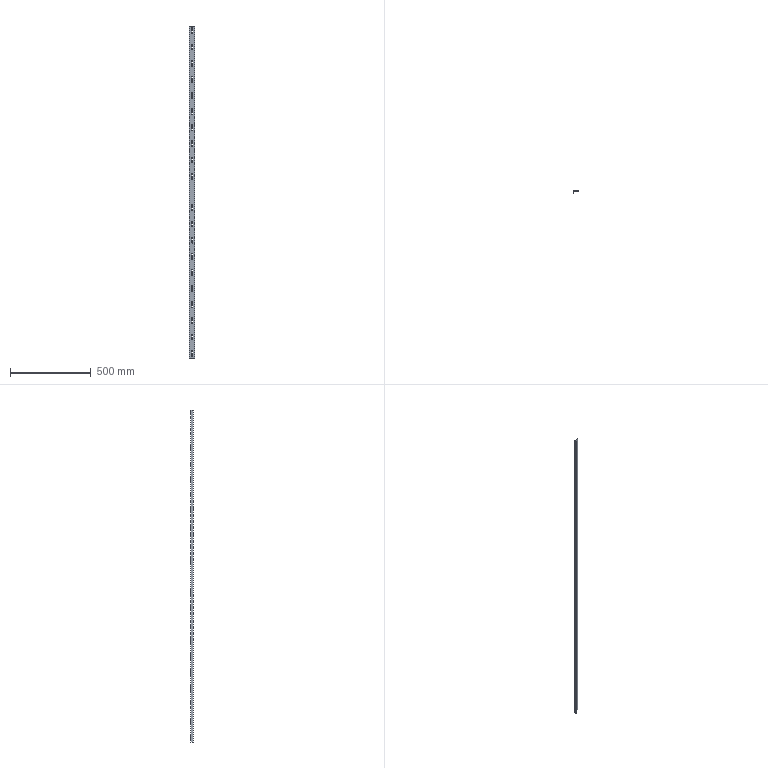Part | SolidWorks | features FlatPattern 1, ICE 1, MirrorPattern 1, SMBaseFlange 1, SheetMetal 1 | 1 solid | 114 faces | box 35 x 18 x 2056 mm | volume 150261 mm3 | cylinder 62 | plane 52 | commonest cylinder face diameters 6 x60 2 x1 5 x1